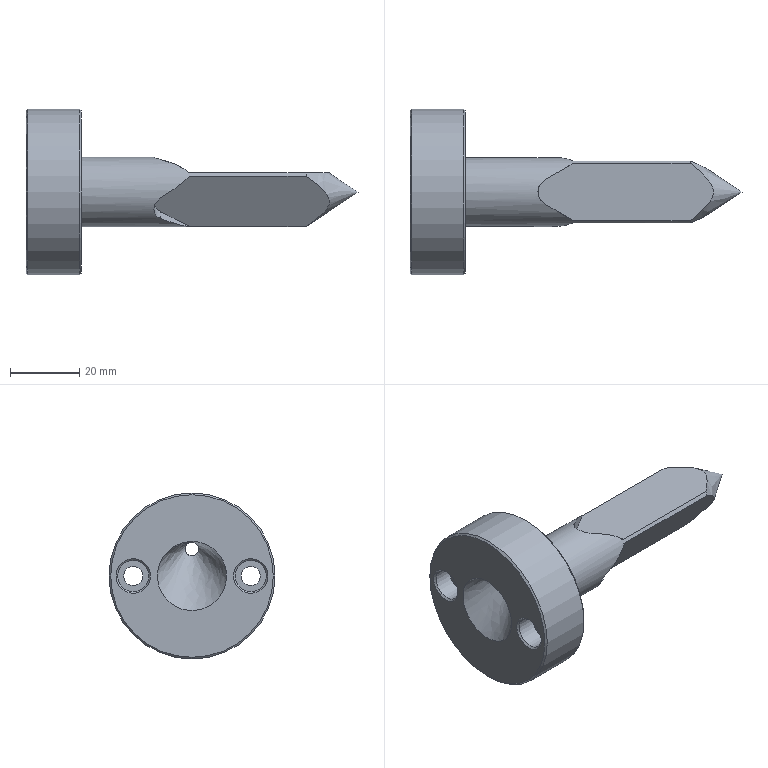NC program | NX | posted with a generic post | part box 96 x 48 x 48 mm
Lines 1796 to 1974 of 1974:
(FLOOR_WALL_COPY , TOOL : D8FINE)
N3578 T09 M6
N3580 G54
N3582 G17 G0 G90 X-75.868 Y-14.352 S5500 M3
N3584 G43 Z31.922 H9
N3586 Z6.5
N3588 G94 G1 Z5.5 F1001.
N3590 X-75.852 Y-13.049
N3592 G3 X-76.243 Y-12.352 R0.8
N3594 G1 X-99.937 Y1.726 F1000.
N3596 Y2.142
N3598 X-96.771 Y4.253
N3600 X-68.823 Y-12.352
N3602 X-61.403
N3604 X-93.274 Y6.584
N3606 X-89.777 Y8.915
N3608 X-53.982 Y-12.352
N3610 X-50.627
N3612 X-51.42 Y-9.465
N3614 X-86.038 Y11.103
N3616 X-85.911 Y11.164
N3618 X-85.041 Y11.56
N3620 X-83.729 Y12.121
N3622 X-83.164 Y12.352
N3624 X-80.72
N3626 X-50.825 Y-5.41
N3628 X-47.115 Y-3.205
N3630 X-73.299 Y12.352
N3632 X-65.879
N3634 X-43.405 Y-1.001
N3636 X-41.72 Y0.
N3638 X-52.032 Y6.127
N3640 G2 X-52.214 Y6.576 R0.4
N3642 G1 X-51.726 Y8.352
N3644 X-58.458 Y12.352
N3646 G3 X-59.258 Y12.362 R0.8
N3648 G1 Y14.352
N3650 Z6.5
N3652 G0 Z13.
N3654 X-51.625 Y-14.352
N3656 Z6.5
N3658 G1 Z5.5 F1001.
N3660 X-50.414 Y-13.126
N3662 G3 X-50.212 Y-12.352 R0.8
N3664 G1 X-51.828 Y-6.47 F1000.
N3666 X-40.937 Y0.
N3668 X-51.828 Y6.471
N3670 X-50.213 Y12.352
N3672 G3 X-50.415 Y13.126 R0.8
N3674 G1 X-51.625 Y14.352
N3676 Z6.5
N3678 G0 Z31.922
(FLOOR_WALL_COPY_COPY , TOOL : D8FINE)
N3680 X-75.868 Y34.821
N3682 Z-3.532
N3684 Y12.805 Z9.179
N3686 G1 Y11.939 Z9.679 F1001.
N3688 X-75.852 Y11.288 Z8.551
N3690 X-75.888 Y11.149 Z8.311
N3692 X-76.025 Y11.026 Z8.098
N3694 X-76.243 Y10.939 Z7.947
N3696 X-99.937 Y3.9 Z-4.245 F1000.
N3698 Y3.692 Z-4.605
N3700 X-96.771 Y2.637 Z-6.433
N3702 X-68.823 Y10.939 Z7.947
N3704 X-61.403
N3706 X-93.274 Y1.471 Z-8.452
N3708 X-89.777 Y0.306 Z-10.471
N3710 X-53.982 Y10.939 Z7.947
N3712 X-50.627
N3714 X-51.42 Y9.496 Z5.447
N3716 X-86.038 Y-0.788 Z-12.365
N3718 X-85.911 Y-0.819 Z-12.419
N3720 X-85.041 Y-1.017 Z-12.761
N3722 X-83.729 Y-1.297 Z-13.247
N3724 X-83.164 Y-1.413 Z-13.447
N3726 X-80.72
N3728 X-50.825 Y7.468 Z1.935
N3730 X-47.115 Y6.366 Z0.026
N3732 X-73.299 Y-1.413 Z-13.447
N3734 X-65.879
N3736 X-43.405 Y5.264 Z-1.883
N3738 X-41.72 Y4.763 Z-2.75
N3740 X-52.032 Y1.7 Z-8.056
N3742 X-52.166 Y1.644 Z-8.153
N3744 X-52.232 Y1.562 Z-8.295
N3746 X-52.214 Y1.475 Z-8.445
N3748 X-51.726 Y0.587 Z-9.983
N3750 X-58.458 Y-1.413 Z-13.447
N3752 X-58.716 Y-1.467 Z-13.54
N3754 X-58.998 Y-1.468 Z-13.544
N3756 X-59.258 Y-1.418 Z-13.456
N3758 Y-2.413 Z-15.179
N3760 Y-1.547 Z-15.679
N3762 G0 Y4.083 Z-18.929
N3764 X-51.625 Y18.434 Z5.929
N3766 Y12.805 Z9.179
N3768 G1 Y11.939 Z9.679 F1001.
N3770 X-50.414 Y11.326 Z8.617
N3772 X-50.247 Y11.214 Z8.423
N3774 X-50.176 Y11.078 Z8.187
N3776 X-50.212 Y10.939 Z7.947
N3778 X-51.828 Y7.998 Z2.854 F1000.
N3780 X-40.937 Y4.763 Z-2.75
N3782 X-51.828 Y1.528 Z-8.354
N3784 X-50.213 Y-1.413 Z-13.447
N3786 X-50.177 Y-1.551 Z-13.687
N3788 X-50.248 Y-1.687 Z-13.923
N3790 X-50.415 Y-1.8 Z-14.117
N3792 X-51.625 Y-2.413 Z-15.179
N3794 Y-1.547 Z-15.679
N3796 G0 Y20.47 Z-28.39
(FLOOR_WALL_COPY_COPY_1 , TOOL : D8FINE)
N3798 X-75.868 Y-20.47
N3800 Y1.547 Z-15.679
N3802 G1 Y2.413 Z-15.179 F1001.
N3804 X-75.852 Y1.762 Z-14.051
N3806 X-75.888 Y1.623 Z-13.811
N3808 X-76.025 Y1.5 Z-13.598
N3810 X-76.243 Y1.413 Z-13.447
N3812 X-99.937 Y-5.626 Z-1.255 F1000.
N3814 Y-5.834 Z-0.895
N3816 X-96.771 Y-6.89 Z0.933
N3818 X-68.823 Y1.413 Z-13.447
N3820 X-61.403
N3822 X-93.274 Y-8.055 Z2.952
N3824 X-89.777 Y-9.221 Z4.971
N3826 X-53.982 Y1.413 Z-13.447
N3828 X-50.627
N3830 X-51.42 Y-0.03 Z-10.947
N3832 X-86.038 Y-10.314 Z6.865
N3834 X-85.911 Y-10.345 Z6.919
N3836 X-85.041 Y-10.543 Z7.261
N3838 X-83.729 Y-10.824 Z7.747
N3840 X-83.164 Y-10.939 Z7.947
N3842 X-80.72
N3844 X-50.825 Y-2.058 Z-7.435
N3846 X-47.115 Y-3.16 Z-5.526
N3848 X-73.299 Y-10.939 Z7.947
N3850 X-65.879
N3852 X-43.405 Y-4.263 Z-3.617
N3854 X-41.72 Y-4.763 Z-2.75
N3856 X-52.032 Y-7.826 Z2.556
N3858 X-52.166 Y-7.882 Z2.653
N3860 X-52.232 Y-7.964 Z2.795
N3862 X-52.214 Y-8.051 Z2.945
N3864 X-51.726 Y-8.939 Z4.483
N3866 X-58.458 Y-10.939 Z7.947
N3868 X-58.716 Y-10.993 Z8.04
N3870 X-58.998 Y-10.995 Z8.044
N3872 X-59.258 Y-10.944 Z7.956
N3874 Y-11.939 Z9.679
N3876 Y-12.805 Z9.179
N3878 G0 Y-18.434 Z5.929
N3880 X-51.625 Y-4.082 Z-18.929
N3882 Y1.547 Z-15.679
N3884 G1 Y2.413 Z-15.179 F1001.
N3886 X-50.414 Y1.8 Z-14.117
N3888 X-50.247 Y1.688 Z-13.923
N3890 X-50.176 Y1.551 Z-13.687
N3892 X-50.212 Y1.413 Z-13.447
N3894 X-51.828 Y-1.528 Z-8.354 F1000.
N3896 X-40.937 Y-4.763 Z-2.75
N3898 X-51.828 Y-7.998 Z2.854
N3900 X-50.213 Y-10.939 Z7.947
N3902 X-50.177 Y-11.078 Z8.187
N3904 X-50.248 Y-11.214 Z8.423
N3906 X-50.415 Y-11.326 Z8.617
N3908 X-51.625 Y-11.939 Z9.679
N3910 Y-12.805 Z9.179
N3912 G0 Y-34.821 Z-3.532
N3914 M5
N3916 M2